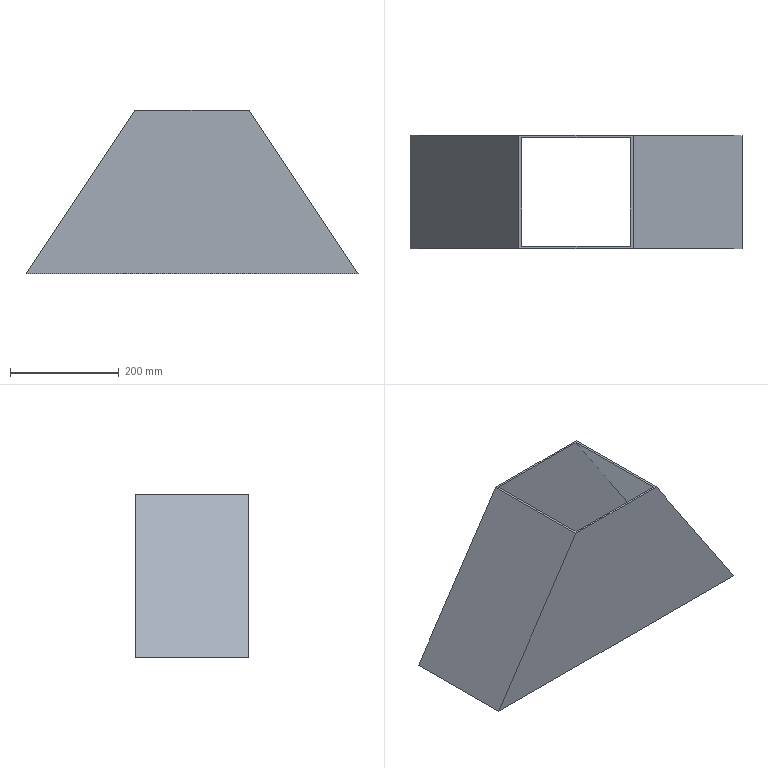Part | SolidWorks | features Blend 1 | 1 solid | 10 faces | box 609.615 x 208 x 300 mm | volume 1559964 mm3 | plane 10
STEP:
#1=CARTESIAN_POINT('',(-304.807,104.,0.));
#2=VERTEX_POINT('',#1);
#3=CARTESIAN_POINT('',(-304.807,-104.,0.));
#4=VERTEX_POINT('',#3);
#5=CARTESIAN_POINT('',(-304.807,0.,0.));
#6=DIRECTION('',(0.,-1.,0.));
#7=VECTOR('',#6,1000.);
#8=LINE('',#5,#7);
#9=EDGE_CURVE('',#2,#4,#8,.T.);
#10=ORIENTED_EDGE('',*,*,#9,.F.);
#11=CARTESIAN_POINT('',(304.807,104.,0.));
#12=VERTEX_POINT('',#11);
#13=CARTESIAN_POINT('',(0.,104.,0.));
#14=DIRECTION('',(-1.,0.,0.));
#15=VECTOR('',#14,1000.);
#16=LINE('',#13,#15);
#17=EDGE_CURVE('',#12,#2,#16,.T.);
#18=ORIENTED_EDGE('',*,*,#17,.F.);
#19=CARTESIAN_POINT('',(304.807,-104.,0.));
#20=VERTEX_POINT('',#19);
#21=CARTESIAN_POINT('',(304.807,0.,0.));
#22=DIRECTION('',(0.,1.,0.));
#23=VECTOR('',#22,1000.);
#24=LINE('',#21,#23);
#25=EDGE_CURVE('',#20,#12,#24,.T.);
#26=ORIENTED_EDGE('',*,*,#25,.F.);
#27=CARTESIAN_POINT('',(0.,-104.,0.));
#28=DIRECTION('',(1.,0.,0.));
#29=VECTOR('',#28,1000.);
#30=LINE('',#27,#29);
#31=EDGE_CURVE('',#4,#20,#30,.T.);
#32=ORIENTED_EDGE('',*,*,#31,.F.);
#33=EDGE_LOOP('',(#10,#18,#26,#32));
#34=FACE_OUTER_BOUND('',#33,.T.);
#35=CARTESIAN_POINT('',(-300.,100.,0.));
#36=VERTEX_POINT('',#35);
#37=CARTESIAN_POINT('',(-300.,-100.,0.));
#38=VERTEX_POINT('',#37);
#39=CARTESIAN_POINT('',(-300.,-100.,0.));
#40=DIRECTION('',(0.,-1.,0.));
#41=VECTOR('',#40,1000.);
#42=LINE('',#39,#41);
#43=EDGE_CURVE('',#36,#38,#42,.T.);
#44=ORIENTED_EDGE('',*,*,#43,.T.);
#45=CARTESIAN_POINT('',(300.,-100.,0.));
#46=VERTEX_POINT('',#45);
#47=CARTESIAN_POINT('',(300.,-100.,0.));
#48=DIRECTION('',(1.,0.,0.));
#49=VECTOR('',#48,1000.);
#50=LINE('',#47,#49);
#51=EDGE_CURVE('',#38,#46,#50,.T.);
#52=ORIENTED_EDGE('',*,*,#51,.T.);
#53=CARTESIAN_POINT('',(300.,100.,0.));
#54=VERTEX_POINT('',#53);
#55=CARTESIAN_POINT('',(300.,-100.,0.));
#56=DIRECTION('',(0.,1.,0.));
#57=VECTOR('',#56,1000.);
#58=LINE('',#55,#57);
#59=EDGE_CURVE('',#46,#54,#58,.T.);
#60=ORIENTED_EDGE('',*,*,#59,.T.);
#61=CARTESIAN_POINT('',(300.,100.,0.));
#62=DIRECTION('',(-1.,0.,0.));
#63=VECTOR('',#62,1000.);
#64=LINE('',#61,#63);
#65=EDGE_CURVE('',#54,#36,#64,.T.);
#66=ORIENTED_EDGE('',*,*,#65,.T.);
#67=EDGE_LOOP('',(#44,#52,#60,#66));
#68=FACE_BOUND('',#67,.T.);
#69=CARTESIAN_POINT('',(0.,0.,0.));
#70=DIRECTION('',(0.,0.,1.));
#71=DIRECTION('',(1.,0.,0.));
#72=AXIS2_PLACEMENT_3D('',#69,#70,#71);
#73=PLANE('',#72);
#74=ADVANCED_FACE('',(#34,#68),#73,.F.);
#75=CARTESIAN_POINT('',(-100.,100.,300.));
#76=VERTEX_POINT('',#75);
#77=CARTESIAN_POINT('',(-100.,-100.,300.));
#78=VERTEX_POINT('',#77);
#79=CARTESIAN_POINT('',(-100.,-100.,300.));
#80=DIRECTION('',(0.,-1.,0.));
#81=VECTOR('',#80,1000.);
#82=LINE('',#79,#81);
#83=EDGE_CURVE('',#76,#78,#82,.T.);
#84=ORIENTED_EDGE('',*,*,#83,.F.);
#85=CARTESIAN_POINT('',(100.,100.,300.));
#86=VERTEX_POINT('',#85);
#87=CARTESIAN_POINT('',(100.,100.,300.));
#88=DIRECTION('',(-1.,0.,0.));
#89=VECTOR('',#88,1000.);
#90=LINE('',#87,#89);
#91=EDGE_CURVE('',#86,#76,#90,.T.);
#92=ORIENTED_EDGE('',*,*,#91,.F.);
#93=CARTESIAN_POINT('',(100.,-100.,300.));
#94=VERTEX_POINT('',#93);
#95=CARTESIAN_POINT('',(100.,-100.,300.));
#96=DIRECTION('',(0.,1.,0.));
#97=VECTOR('',#96,1000.);
#98=LINE('',#95,#97);
#99=EDGE_CURVE('',#94,#86,#98,.T.);
#100=ORIENTED_EDGE('',*,*,#99,.F.);
#101=CARTESIAN_POINT('',(100.,-100.,300.));
#102=DIRECTION('',(1.,0.,0.));
#103=VECTOR('',#102,1000.);
#104=LINE('',#101,#103);
#105=EDGE_CURVE('',#78,#94,#104,.T.);
#106=ORIENTED_EDGE('',*,*,#105,.F.);
#107=EDGE_LOOP('',(#84,#92,#100,#106));
#108=FACE_BOUND('',#107,.T.);
#109=CARTESIAN_POINT('',(-104.807,104.,300.));
#110=VERTEX_POINT('',#109);
#111=CARTESIAN_POINT('',(-104.807,-104.,300.));
#112=VERTEX_POINT('',#111);
#113=CARTESIAN_POINT('',(-104.807,0.,300.));
#114=DIRECTION('',(0.,-1.,0.));
#115=VECTOR('',#114,1000.);
#116=LINE('',#113,#115);
#117=EDGE_CURVE('',#110,#112,#116,.T.);
#118=ORIENTED_EDGE('',*,*,#117,.T.);
#119=CARTESIAN_POINT('',(104.807,-104.,300.));
#120=VERTEX_POINT('',#119);
#121=CARTESIAN_POINT('',(0.,-104.,300.));
#122=DIRECTION('',(1.,0.,0.));
#123=VECTOR('',#122,1000.);
#124=LINE('',#121,#123);
#125=EDGE_CURVE('',#112,#120,#124,.T.);
#126=ORIENTED_EDGE('',*,*,#125,.T.);
#127=CARTESIAN_POINT('',(104.807,104.,300.));
#128=VERTEX_POINT('',#127);
#129=CARTESIAN_POINT('',(104.807,0.,300.));
#130=DIRECTION('',(0.,1.,0.));
#131=VECTOR('',#130,1000.);
#132=LINE('',#129,#131);
#133=EDGE_CURVE('',#120,#128,#132,.T.);
#134=ORIENTED_EDGE('',*,*,#133,.T.);
#135=CARTESIAN_POINT('',(0.,104.,300.));
#136=DIRECTION('',(-1.,0.,0.));
#137=VECTOR('',#136,1000.);
#138=LINE('',#135,#137);
#139=EDGE_CURVE('',#128,#110,#138,.T.);
#140=ORIENTED_EDGE('',*,*,#139,.T.);
#141=EDGE_LOOP('',(#118,#126,#134,#140));
#142=FACE_OUTER_BOUND('',#141,.T.);
#143=CARTESIAN_POINT('',(0.,0.,300.));
#144=DIRECTION('',(0.,0.,1.));
#145=DIRECTION('',(1.,0.,0.));
#146=AXIS2_PLACEMENT_3D('',#143,#144,#145);
#147=PLANE('',#146);
#148=ADVANCED_FACE('',(#108,#142),#147,.T.);
#149=CARTESIAN_POINT('',(211.021,-104.,140.68));
#150=DIRECTION('',(0.5547,0.,-0.8321));
#151=VECTOR('',#150,1000.);
#152=LINE('',#149,#151);
#153=EDGE_CURVE('',#120,#20,#152,.T.);
#154=ORIENTED_EDGE('',*,*,#153,.T.);
#155=ORIENTED_EDGE('',*,*,#25,.T.);
#156=CARTESIAN_POINT('',(211.021,104.,140.68));
#157=DIRECTION('',(0.5547,0.,-0.8321));
#158=VECTOR('',#157,1000.);
#159=LINE('',#156,#158);
#160=EDGE_CURVE('',#128,#12,#159,.T.);
#161=ORIENTED_EDGE('',*,*,#160,.F.);
#162=ORIENTED_EDGE('',*,*,#133,.F.);
#163=EDGE_LOOP('',(#154,#155,#161,#162));
#164=FACE_OUTER_BOUND('',#163,.T.);
#165=CARTESIAN_POINT('',(211.021,0.,140.68));
#166=DIRECTION('',(0.8321,0.,0.5547));
#167=DIRECTION('',(0.5547,0.,-0.8321));
#168=AXIS2_PLACEMENT_3D('',#165,#166,#167);
#169=PLANE('',#168);
#170=ADVANCED_FACE('',(#164),#169,.T.);
#171=ORIENTED_EDGE('',*,*,#160,.T.);
#172=ORIENTED_EDGE('',*,*,#17,.T.);
#173=CARTESIAN_POINT('',(-211.021,104.,140.68));
#174=DIRECTION('',(-0.5547,0.,-0.8321));
#175=VECTOR('',#174,1000.);
#176=LINE('',#173,#175);
#177=EDGE_CURVE('',#110,#2,#176,.T.);
#178=ORIENTED_EDGE('',*,*,#177,.F.);
#179=ORIENTED_EDGE('',*,*,#139,.F.);
#180=EDGE_LOOP('',(#171,#172,#178,#179));
#181=FACE_OUTER_BOUND('',#180,.T.);
#182=CARTESIAN_POINT('',(0.,104.,0.));
#183=DIRECTION('',(0.,1.,0.));
#184=DIRECTION('',(-1.,0.,0.));
#185=AXIS2_PLACEMENT_3D('',#182,#183,#184);
#186=PLANE('',#185);
#187=ADVANCED_FACE('',(#181),#186,.T.);
#188=CARTESIAN_POINT('',(-211.021,-104.,140.68));
#189=DIRECTION('',(-0.5547,0.,-0.8321));
#190=VECTOR('',#189,1000.);
#191=LINE('',#188,#190);
#192=EDGE_CURVE('',#112,#4,#191,.T.);
#193=ORIENTED_EDGE('',*,*,#192,.T.);
#194=ORIENTED_EDGE('',*,*,#31,.T.);
#195=ORIENTED_EDGE('',*,*,#153,.F.);
#196=ORIENTED_EDGE('',*,*,#125,.F.);
#197=EDGE_LOOP('',(#193,#194,#195,#196));
#198=FACE_OUTER_BOUND('',#197,.T.);
#199=CARTESIAN_POINT('',(0.,-104.,0.));
#200=DIRECTION('',(0.,-1.,0.));
#201=DIRECTION('',(1.,0.,0.));
#202=AXIS2_PLACEMENT_3D('',#199,#200,#201);
#203=PLANE('',#202);
#204=ADVANCED_FACE('',(#198),#203,.T.);
#205=ORIENTED_EDGE('',*,*,#177,.T.);
#206=ORIENTED_EDGE('',*,*,#9,.T.);
#207=ORIENTED_EDGE('',*,*,#192,.F.);
#208=ORIENTED_EDGE('',*,*,#117,.F.);
#209=EDGE_LOOP('',(#205,#206,#207,#208));
#210=FACE_OUTER_BOUND('',#209,.T.);
#211=CARTESIAN_POINT('',(-211.021,0.,140.68));
#212=DIRECTION('',(-0.8321,0.,0.5547));
#213=DIRECTION('',(0.5547,0.,0.8321));
#214=AXIS2_PLACEMENT_3D('',#211,#212,#213);
#215=PLANE('',#214);
#216=ADVANCED_FACE('',(#210),#215,.T.);
#217=CARTESIAN_POINT('',(100.,-100.,300.));
#218=DIRECTION('',(0.5547,0.,-0.8321));
#219=VECTOR('',#218,1000.);
#220=LINE('',#217,#219);
#221=EDGE_CURVE('',#94,#46,#220,.T.);
#222=ORIENTED_EDGE('',*,*,#221,.F.);
#223=ORIENTED_EDGE('',*,*,#99,.T.);
#224=CARTESIAN_POINT('',(100.,100.,300.));
#225=DIRECTION('',(0.5547,0.,-0.8321));
#226=VECTOR('',#225,1000.);
#227=LINE('',#224,#226);
#228=EDGE_CURVE('',#86,#54,#227,.T.);
#229=ORIENTED_EDGE('',*,*,#228,.T.);
#230=ORIENTED_EDGE('',*,*,#59,.F.);
#231=EDGE_LOOP('',(#222,#223,#229,#230));
#232=FACE_OUTER_BOUND('',#231,.T.);
#233=CARTESIAN_POINT('',(207.692,0.,138.462));
#234=DIRECTION('',(0.8321,0.,0.5547));
#235=DIRECTION('',(0.5547,0.,-0.8321));
#236=AXIS2_PLACEMENT_3D('',#233,#234,#235);
#237=PLANE('',#236);
#238=ADVANCED_FACE('',(#232),#237,.F.);
#239=ORIENTED_EDGE('',*,*,#228,.F.);
#240=ORIENTED_EDGE('',*,*,#91,.T.);
#241=CARTESIAN_POINT('',(-100.,100.,300.));
#242=DIRECTION('',(-0.5547,0.,-0.8321));
#243=VECTOR('',#242,1000.);
#244=LINE('',#241,#243);
#245=EDGE_CURVE('',#76,#36,#244,.T.);
#246=ORIENTED_EDGE('',*,*,#245,.T.);
#247=ORIENTED_EDGE('',*,*,#65,.F.);
#248=EDGE_LOOP('',(#239,#240,#246,#247));
#249=FACE_OUTER_BOUND('',#248,.T.);
#250=CARTESIAN_POINT('',(0.,100.,0.));
#251=DIRECTION('',(0.,1.,0.));
#252=DIRECTION('',(-1.,0.,0.));
#253=AXIS2_PLACEMENT_3D('',#250,#251,#252);
#254=PLANE('',#253);
#255=ADVANCED_FACE('',(#249),#254,.F.);
#256=CARTESIAN_POINT('',(-100.,-100.,300.));
#257=DIRECTION('',(-0.5547,0.,-0.8321));
#258=VECTOR('',#257,1000.);
#259=LINE('',#256,#258);
#260=EDGE_CURVE('',#78,#38,#259,.T.);
#261=ORIENTED_EDGE('',*,*,#260,.F.);
#262=ORIENTED_EDGE('',*,*,#105,.T.);
#263=ORIENTED_EDGE('',*,*,#221,.T.);
#264=ORIENTED_EDGE('',*,*,#51,.F.);
#265=EDGE_LOOP('',(#261,#262,#263,#264));
#266=FACE_OUTER_BOUND('',#265,.T.);
#267=CARTESIAN_POINT('',(0.,-100.,0.));
#268=DIRECTION('',(0.,-1.,0.));
#269=DIRECTION('',(1.,0.,0.));
#270=AXIS2_PLACEMENT_3D('',#267,#268,#269);
#271=PLANE('',#270);
#272=ADVANCED_FACE('',(#266),#271,.F.);
#273=ORIENTED_EDGE('',*,*,#245,.F.);
#274=ORIENTED_EDGE('',*,*,#83,.T.);
#275=ORIENTED_EDGE('',*,*,#260,.T.);
#276=ORIENTED_EDGE('',*,*,#43,.F.);
#277=EDGE_LOOP('',(#273,#274,#275,#276));
#278=FACE_OUTER_BOUND('',#277,.T.);
#279=CARTESIAN_POINT('',(-207.692,0.,138.462));
#280=DIRECTION('',(-0.8321,0.,0.5547));
#281=DIRECTION('',(0.5547,0.,0.8321));
#282=AXIS2_PLACEMENT_3D('',#279,#280,#281);
#283=PLANE('',#282);
#284=ADVANCED_FACE('',(#278),#283,.F.);
#285=CLOSED_SHELL('',(#74,#148,#170,#187,#204,#216,#238,#255,#272,#284));
#286=MANIFOLD_SOLID_BREP('',#285);
#287=CARTESIAN_POINT('',(0.,0.,0.));
#288=DIRECTION('',(0.,0.,1.));
#289=DIRECTION('',(1.,0.,0.));
#290=AXIS2_PLACEMENT_3D('',#287,#288,#289);
#291=(LENGTH_UNIT()NAMED_UNIT(*)SI_UNIT(.MILLI.,.METRE.));
#292=UNCERTAINTY_MEASURE_WITH_UNIT(LENGTH_MEASURE(0.00001),#291,'','');
#293=(NAMED_UNIT(*)PLANE_ANGLE_UNIT()SI_UNIT($,.RADIAN.));
#294=(NAMED_UNIT(*)SI_UNIT($,.STERADIAN.)SOLID_ANGLE_UNIT());
#295=(GEOMETRIC_REPRESENTATION_CONTEXT(3)GLOBAL_UNCERTAINTY_ASSIGNED_CONTEXT((#292))GLOBAL_UNIT_ASSIGNED_CONTEXT((#291,#293,#294))REPRESENTATION_CONTEXT('',''));
#296=ADVANCED_BREP_SHAPE_REPRESENTATION('',(#286,#290),#295);